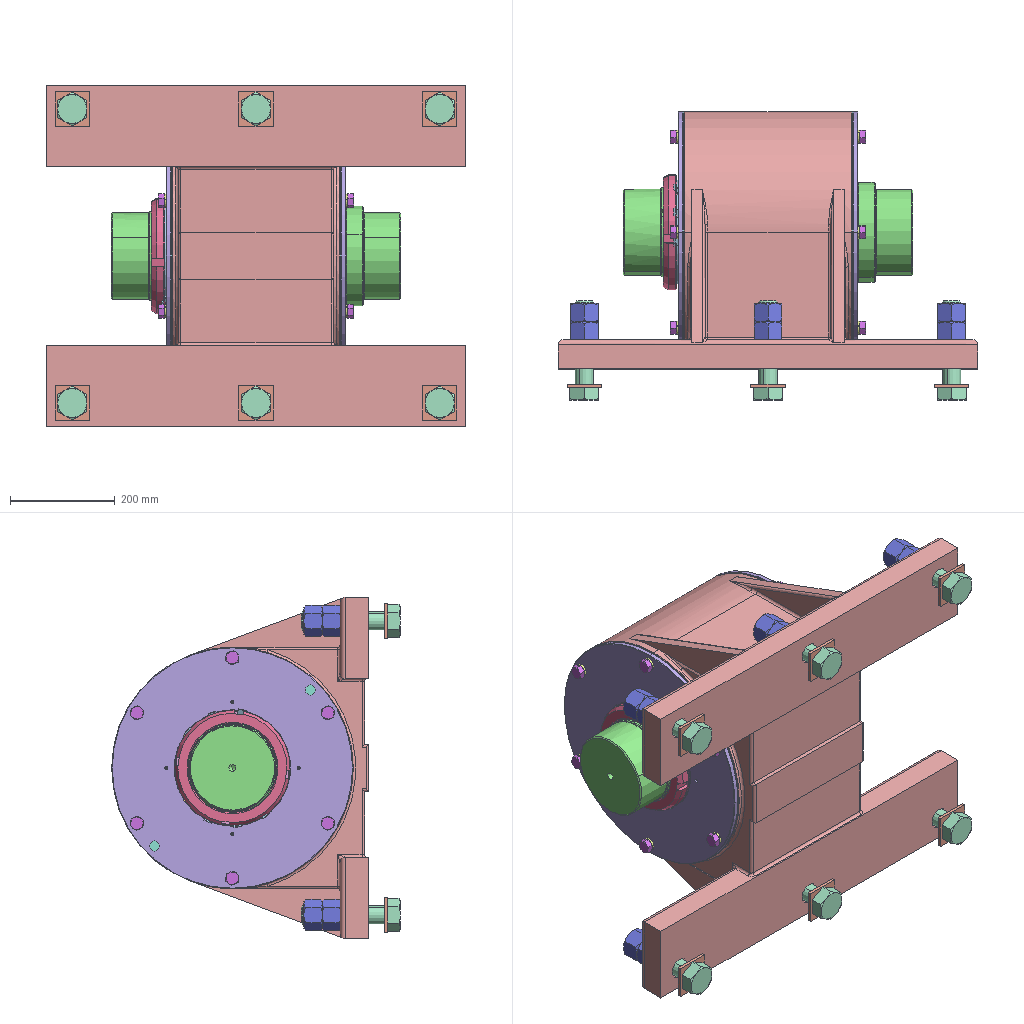Assembly | SolidWorks | 16 different items | 64 placed | box 800 x 550 x 650 mm
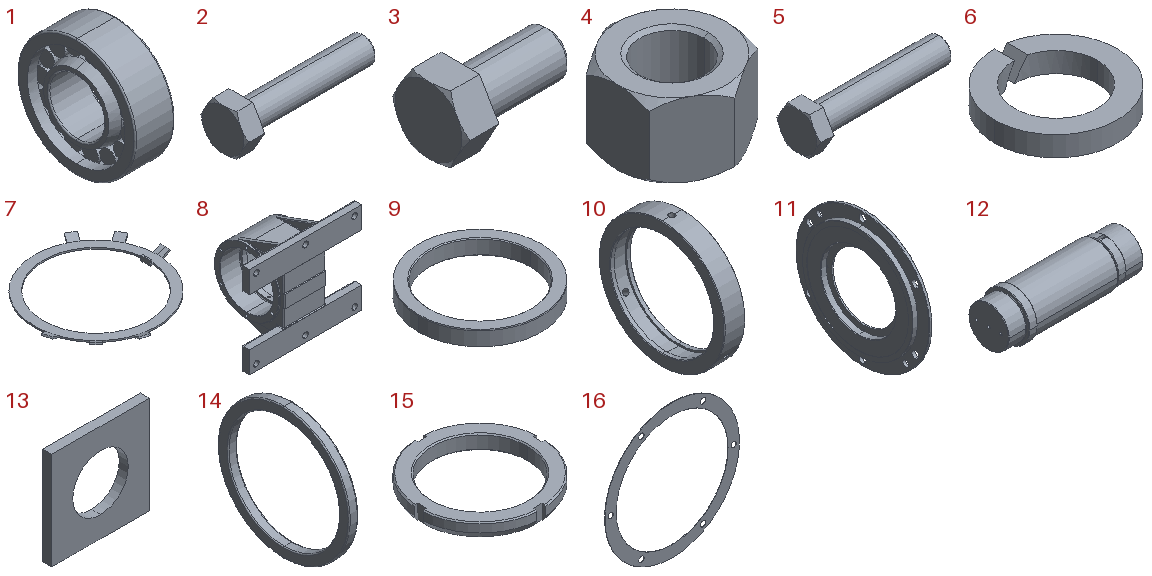Parts list (item | quantity | size | volume | features):
1 | x2 | 114 x 340 x 340 mm | 5597424 mm3 | features Revolution 3, Fillet 2, CirPattern 1
2 | x6 | 188.976 x 64.173 x 55.575 mm | 221511 mm3 | features RevCut 2, Extrusion 1, Fillet 1, LPattern 1, Revolution 1
3 | x12 | 25.857 x 16.483 x 14.275 mm | 2543 mm3 | features RevCut 2, Extrusion 1, Fillet 1, LPattern 1, Revolution 1
4 | x12 | 52.375 x 60.477 x 35.535 mm | 56919 mm3 | features RevCut 4, Extrusion 1, LPattern 1
5 | x1 | 67.5 x 20.785 x 18 mm | 8849 mm3 | features RevCut 3, Boss 1, Chamfer 1, Extrusion 1, Fillet 1, LPattern 1
6 | x12 | 22.1 x 22.1 x 3.6 mm | 726.172 mm3 | features Cut 1, Extrusion 1
7 | x1 | 223.898 x 212.404 x 8.087 mm | 24578 mm3 | features Boss 1, Cut 1, Revolution 1
8 | x1 | 800 x 490 x 650 mm | 39850758 mm3 | features ICE 6, Fillet 4, MirrorPattern 3, 3DProfileFeature 2, HoleWzd 2, LPattern 2, Chamfer 1, CirPattern 1, Revolution 1
9 | x2 | 220 x 220 x 27 mm | 337527 mm3 | features Chamfer 2, Extrusion 1
10 | x1 | 36 x 220 x 220 mm | 409173 mm3 | features 3DProfileFeature 1, Chamfer 1, CirPattern 1, HoleWzd 1, Revolution 1
11 | x2 | 27 x 460 x 460 mm | 2105445 mm3 | features ICE 4, CirPattern 3, Chamfer 2, 3DProfileFeature 1, HoleWzd 1, Revolution 1
12 | x1 | 552 x 191 x 191 mm | 13392026 mm3 | features HoleWzd 4, Fillet 3, Chamfer 2, ICE 2, Revolution 1
13 | x6 | 65 x 6 x 65 mm | 18899 mm3 | features Extrusion 1
14 | x2 | 18 x 260 x 260 mm | 189235 mm3 | features Revolution 1
15 | x1 | 219.417 x 219.417 x 26 mm | 365558 mm3 | features Chamfer 3, ICE 2, Extrusion 1
16 | x2 | 460 x 1 x 460 mm | 50055 mm3 | features CirPattern 1, Extrusion 1, ICE 1
Mates (type | each side: item.copy, entity, surface, feature):
Coincident | 8.1 plane | assembly plane | 3 times
Concentric | 8.1 face cylinder Revolve1 | 1.1 face cylinder Revolve3
Concentric | 1.2 face cylinder Revolve3 | 10.1 face cylinder Revolve1
Concentric | 8.1 face cylinder Revolve1 | 9.1 face cylinder Boss-Extrude1
Coincident | 9.1 face plane Boss-Extrude1 | 12.1 face plane Revolve1
Concentric | 8.1 face cylinder Revolve1 | 16.1 face cylinder Boss-Extrude1
Coincident | 8.1 face plane Revolve1 | 16.1 face plane Boss-Extrude1
Concentric | 8.1 face cylinder CirPattern2 | 16.1 face cylinder CirPattern1
Concentric | 8.1 face cylinder Revolve1 | 14.1 face cylinder Revolve1
DistanceDim | 14.1 face plane Revolve1 | 9.1 face plane Boss-Extrude1
Concentric | 8.1 face cylinder Revolve1 | 11.1 face cylinder Revolve1
Coincident | 16.1 face plane Boss-Extrude1 | 11.1 face plane Revolve1
Concentric | 8.1 face cylinder CirPattern2 | 11.1 face cylinder CirPattern1
Concentric | 8.1 face cylinder Revolve1 | 12.1 face cylinder Revolve1
Coincident | 11.1 face plane Revolve1 | 12.1 face plane Revolve1
Concentric | 8.1 face cylinder Revolve1 | 7.1 face cylinder Cut-Extrude
Coincident | 9.2 face plane Boss-Extrude1 | 7.1 face plane Base-Extrude
Concentric | 8.1 face cylinder Revolve1 | 15.1 face cylinder Boss-Extrude1
Coincident | 15.1 face plane Boss-Extrude1 | 7.1 face plane Base-Extrude
Concentric | 11.1 face cylinder CirPattern1 | 6.1 face cylinder Base-Extrude
Coincident | 11.1 face plane Revolve1 | 6.1 face plane Base-Extrude
Concentric | 11.1 face cylinder CirPattern1 | 3.1 face cylinder BaseBody
Coincident | 6.1 face plane Base-Extrude | 3.1 face plane BaseHead
Concentric | 8.1 face cylinder LPattern1 | 13.1 face cylinder Boss-Extrude1
DistanceDim | 13.1 face plane Boss-Extrude1 | 8.1 face plane Boss-Extrude1
Concentric | 8.1 face cylinder LPattern1 | 2.1 face cylinder BaseBody
Coincident | 2.1 face plane BaseHead | 13.1 face plane Boss-Extrude1
Parallel | 2.1 face plane BaseHead | 13.1 face plane Boss-Extrude1
Parallel | 13.1 face plane Boss-Extrude1 | 8.1 face plane Boss-Extrude2
Concentric | 2.1 face cylinder BaseBody | 4.1 face cylinder BaseNut
Coincident | 8.1 face plane LPattern2 | 4.1 face plane BaseNut
Parallel | 2.1 face plane BaseHead | 4.1 face plane BaseNut
Concentric | 2.1 face cylinder BaseBody | 4.2 face cylinder BaseNut
Coincident | 4.1 face plane BaseNut | 4.2 face plane BaseNut | 2 times
Concentric | 8.1 face cylinder ZG1/4 | 5.1 face cylinder BaseBody
Coincident | 8.1 face plane Cut-Extrude5 | 5.1 face plane BaseHead
Coincident | 1.1 face plane Revolve3 | 11.1 face plane Revolve1
Coincident | 10.1 plane | assembly plane